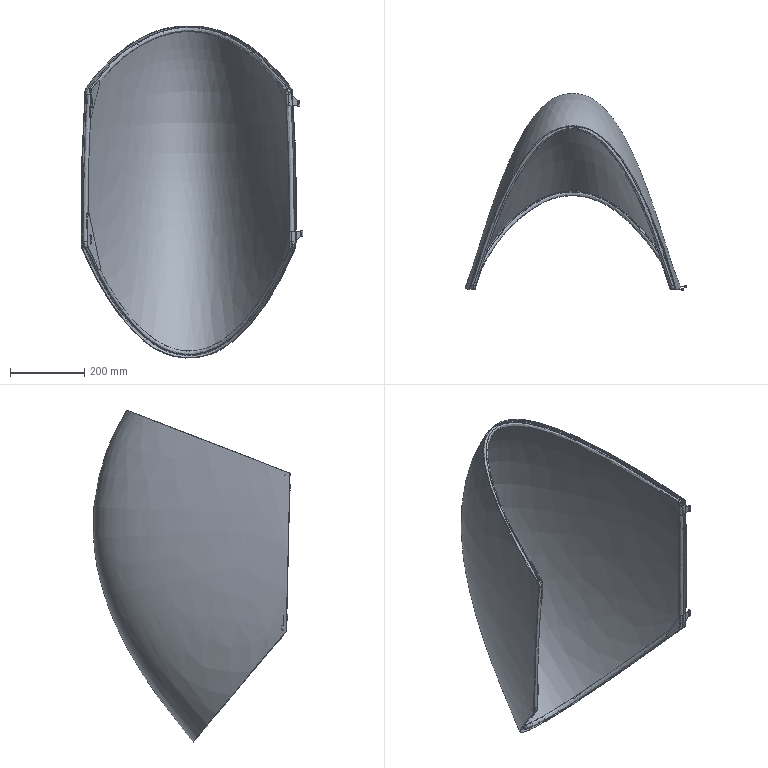Part | SolidWorks | features BaseBody 18 | 18 solids | 132 faces | box 596.838 x 531.655 x 893.834 mm | volume 1963932 mm3 | plane 58 | spline 43 | cylinder 31 | commonest cylinder face diameters 6 x6 12 x6 13 x6 4 x4 6.4 x4 24 x3